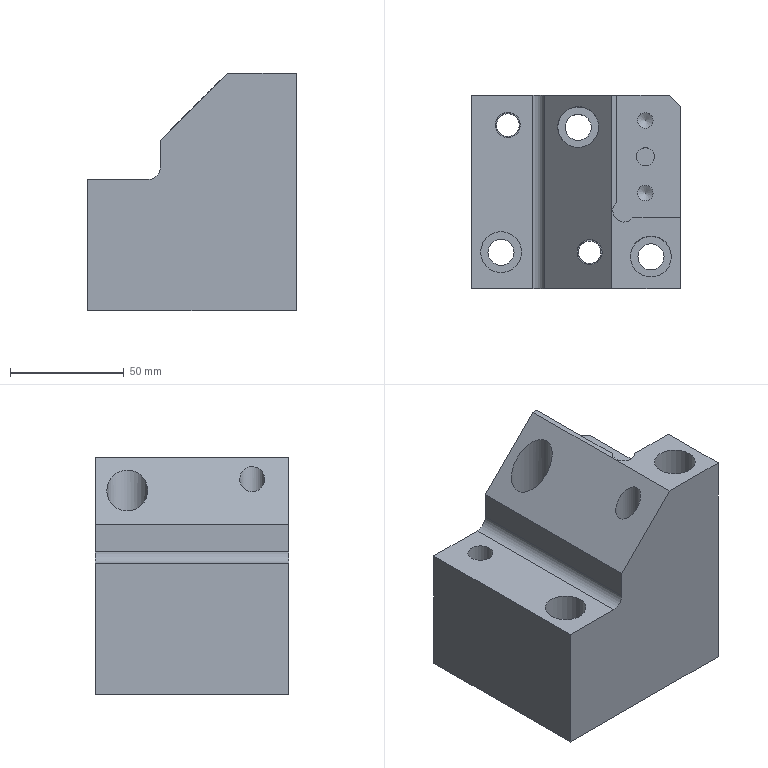Part | NX | features solid 2 | 1 solid | 36 faces | box 92 x 85 x 104.5 mm | volume 547105 mm3 | plane 19 | cylinder 15 | cone 2 | commonest cylinder face diameters 11.5 x3 6.8 x2 10 x2 10.001 x2 11 x2 18.008 x2
STEP:
#1=CARTESIAN_POINT('',(3692.099,-404.,-58.502));
#2=VERTEX_POINT('',#1);
#3=CARTESIAN_POINT('',(3688.699,-404.,-58.502));
#4=DIRECTION('',(0.,0.,1.));
#5=DIRECTION('',(1.,0.,0.));
#6=AXIS2_PLACEMENT_3D('',#3,#4,#5);
#7=CIRCLE('',#6,3.4);
#8=EDGE_CURVE('',#2,#2,#7,.T.);
#9=ORIENTED_EDGE('',*,*,#8,.T.);
#10=EDGE_LOOP('',(#9));
#11=FACE_BOUND('',#10,.T.);
#12=CARTESIAN_POINT('',(3688.699,-404.,-60.545));
#13=VERTEX_POINT('',#12);
#14=VERTEX_LOOP('',#13);
#15=FACE_BOUND('',#14,.T.);
#16=CARTESIAN_POINT('',(3688.699,-404.,-58.5));
#17=DIRECTION('',(0.,0.,1.));
#18=DIRECTION('',(1.,0.,0.));
#19=AXIS2_PLACEMENT_3D('',#16,#17,#18);
#20=CONICAL_SURFACE('',#19,3.403,1.03);
#21=ADVANCED_FACE('',(#11,#15),#20,.F.);
#22=ORIENTED_EDGE('',*,*,#8,.F.);
#23=EDGE_LOOP('',(#22));
#24=FACE_BOUND('',#23,.T.);
#25=CARTESIAN_POINT('',(3685.299,-404.,-33.5));
#26=VERTEX_POINT('',#25);
#27=CARTESIAN_POINT('',(3688.699,-404.,-33.5));
#28=DIRECTION('',(0.,0.,1.));
#29=DIRECTION('',(-1.,0.,0.));
#30=AXIS2_PLACEMENT_3D('',#27,#28,#29);
#31=CIRCLE('',#30,3.4);
#32=EDGE_CURVE('',#26,#26,#31,.T.);
#33=ORIENTED_EDGE('',*,*,#32,.T.);
#34=EDGE_LOOP('',(#33));
#35=FACE_BOUND('',#34,.T.);
#36=CARTESIAN_POINT('',(3688.699,-404.,-33.5));
#37=DIRECTION('',(0.,0.,-1.));
#38=DIRECTION('',(-1.,0.,0.));
#39=AXIS2_PLACEMENT_3D('',#36,#37,#38);
#40=CYLINDRICAL_SURFACE('',#39,3.4);
#41=ADVANCED_FACE('',(#24,#35),#40,.F.);
#42=CARTESIAN_POINT('',(3659.199,-462.,-83.));
#43=VERTEX_POINT('',#42);
#44=CARTESIAN_POINT('',(3664.199,-462.,-83.));
#45=DIRECTION('',(0.,0.,1.));
#46=DIRECTION('',(-1.,0.,0.));
#47=AXIS2_PLACEMENT_3D('',#44,#45,#46);
#48=CIRCLE('',#47,5.);
#49=EDGE_CURVE('',#43,#43,#48,.T.);
#50=ORIENTED_EDGE('',*,*,#49,.F.);
#51=EDGE_LOOP('',(#50));
#52=FACE_BOUND('',#51,.T.);
#53=CARTESIAN_POINT('',(3669.699,-462.,-83.));
#54=VERTEX_POINT('',#53);
#55=CARTESIAN_POINT('',(3664.199,-462.,-83.));
#56=DIRECTION('',(0.,0.,1.));
#57=DIRECTION('',(1.,0.,0.));
#58=AXIS2_PLACEMENT_3D('',#55,#56,#57);
#59=CIRCLE('',#58,5.5);
#60=EDGE_CURVE('',#54,#54,#59,.T.);
#61=ORIENTED_EDGE('',*,*,#60,.T.);
#62=EDGE_LOOP('',(#61));
#63=FACE_BOUND('',#62,.T.);
#64=CARTESIAN_POINT('',(3691.199,-464.,-83.));
#65=DIRECTION('',(0.,0.,-1.));
#66=DIRECTION('',(-1.,0.,0.));
#67=AXIS2_PLACEMENT_3D('',#64,#65,#66);
#68=PLANE('',#67);
#69=ADVANCED_FACE('',(#52,#63),#68,.F.);
#70=CARTESIAN_POINT('',(3682.199,-464.,-83.));
#71=VERTEX_POINT('',#70);
#72=CARTESIAN_POINT('',(3691.199,-464.,-83.));
#73=DIRECTION('',(0.,0.,-1.));
#74=DIRECTION('',(-1.,0.,0.));
#75=AXIS2_PLACEMENT_3D('',#72,#73,#74);
#76=CIRCLE('',#75,9.);
#77=EDGE_CURVE('',#71,#71,#76,.T.);
#78=ORIENTED_EDGE('',*,*,#77,.F.);
#79=EDGE_LOOP('',(#78));
#80=FACE_BOUND('',#79,.T.);
#81=CARTESIAN_POINT('',(3685.449,-464.,-83.));
#82=VERTEX_POINT('',#81);
#83=CARTESIAN_POINT('',(3691.199,-464.,-83.));
#84=DIRECTION('',(0.,0.,-1.));
#85=DIRECTION('',(-1.,0.,0.));
#86=AXIS2_PLACEMENT_3D('',#83,#84,#85);
#87=CIRCLE('',#86,5.75);
#88=EDGE_CURVE('',#82,#82,#87,.T.);
#89=ORIENTED_EDGE('',*,*,#88,.T.);
#90=EDGE_LOOP('',(#89));
#91=FACE_BOUND('',#90,.T.);
#92=CARTESIAN_POINT('',(2606.199,-221.,-83.));
#93=DIRECTION('',(0.,0.,-1.));
#94=DIRECTION('',(-1.,0.,0.));
#95=AXIS2_PLACEMENT_3D('',#92,#93,#94);
#96=PLANE('',#95);
#97=ADVANCED_FACE('',(#80,#91),#96,.F.);
#98=CARTESIAN_POINT('',(3650.195,-407.,-83.));
#99=VERTEX_POINT('',#98);
#100=CARTESIAN_POINT('',(3659.199,-407.,-83.));
#101=DIRECTION('',(0.,0.,-1.));
#102=DIRECTION('',(-1.,0.,0.));
#103=AXIS2_PLACEMENT_3D('',#100,#101,#102);
#104=CIRCLE('',#103,9.004);
#105=EDGE_CURVE('',#99,#99,#104,.T.);
#106=ORIENTED_EDGE('',*,*,#105,.F.);
#107=EDGE_LOOP('',(#106));
#108=FACE_BOUND('',#107,.T.);
#109=CARTESIAN_POINT('',(3653.449,-407.,-83.));
#110=VERTEX_POINT('',#109);
#111=CARTESIAN_POINT('',(3659.199,-407.,-83.));
#112=DIRECTION('',(0.,0.,-1.));
#113=DIRECTION('',(-1.,0.,0.));
#114=AXIS2_PLACEMENT_3D('',#111,#112,#113);
#115=CIRCLE('',#114,5.75);
#116=EDGE_CURVE('',#110,#110,#115,.T.);
#117=ORIENTED_EDGE('',*,*,#116,.T.);
#118=EDGE_LOOP('',(#117));
#119=FACE_BOUND('',#118,.T.);
#120=CARTESIAN_POINT('',(2606.199,-221.,-83.));
#121=DIRECTION('',(0.,0.,-1.));
#122=DIRECTION('',(-1.,0.,0.));
#123=AXIS2_PLACEMENT_3D('',#120,#121,#122);
#124=PLANE('',#123);
#125=ADVANCED_FACE('',(#108,#119),#124,.F.);
#126=CARTESIAN_POINT('',(3623.199,-406.,-83.));
#127=VERTEX_POINT('',#126);
#128=CARTESIAN_POINT('',(3628.199,-406.,-83.));
#129=DIRECTION('',(0.,0.,1.));
#130=DIRECTION('',(-1.,0.,0.));
#131=AXIS2_PLACEMENT_3D('',#128,#129,#130);
#132=CIRCLE('',#131,5.);
#133=EDGE_CURVE('',#127,#127,#132,.T.);
#134=ORIENTED_EDGE('',*,*,#133,.F.);
#135=EDGE_LOOP('',(#134));
#136=FACE_BOUND('',#135,.T.);
#137=CARTESIAN_POINT('',(3633.699,-406.,-83.));
#138=VERTEX_POINT('',#137);
#139=CARTESIAN_POINT('',(3628.199,-406.,-83.));
#140=DIRECTION('',(0.,0.,1.));
#141=DIRECTION('',(1.,0.,0.));
#142=AXIS2_PLACEMENT_3D('',#139,#140,#141);
#143=CIRCLE('',#142,5.5);
#144=EDGE_CURVE('',#138,#138,#143,.T.);
#145=ORIENTED_EDGE('',*,*,#144,.T.);
#146=EDGE_LOOP('',(#145));
#147=FACE_BOUND('',#146,.T.);
#148=CARTESIAN_POINT('',(3660.199,-443.,-83.));
#149=DIRECTION('',(0.,0.,-1.));
#150=DIRECTION('',(-1.,0.,0.));
#151=AXIS2_PLACEMENT_3D('',#148,#149,#150);
#152=PLANE('',#151);
#153=ADVANCED_FACE('',(#136,#147),#152,.F.);
#154=CARTESIAN_POINT('',(3616.195,-462.,-83.));
#155=VERTEX_POINT('',#154);
#156=CARTESIAN_POINT('',(3625.199,-462.,-83.));
#157=DIRECTION('',(0.,0.,-1.));
#158=DIRECTION('',(-1.,0.,0.));
#159=AXIS2_PLACEMENT_3D('',#156,#157,#158);
#160=CIRCLE('',#159,9.004);
#161=EDGE_CURVE('',#155,#155,#160,.T.);
#162=ORIENTED_EDGE('',*,*,#161,.F.);
#163=EDGE_LOOP('',(#162));
#164=FACE_BOUND('',#163,.T.);
#165=CARTESIAN_POINT('',(3619.449,-462.,-83.));
#166=VERTEX_POINT('',#165);
#167=CARTESIAN_POINT('',(3625.199,-462.,-83.));
#168=DIRECTION('',(0.,0.,-1.));
#169=DIRECTION('',(-1.,0.,0.));
#170=AXIS2_PLACEMENT_3D('',#167,#168,#169);
#171=CIRCLE('',#170,5.75);
#172=EDGE_CURVE('',#166,#166,#171,.T.);
#173=ORIENTED_EDGE('',*,*,#172,.T.);
#174=EDGE_LOOP('',(#173));
#175=FACE_BOUND('',#174,.T.);
#176=CARTESIAN_POINT('',(2606.199,-238.,-83.));
#177=DIRECTION('',(0.,0.,-1.));
#178=DIRECTION('',(-1.,0.,0.));
#179=AXIS2_PLACEMENT_3D('',#176,#177,#178);
#180=PLANE('',#179);
#181=ADVANCED_FACE('',(#164,#175),#180,.F.);
#182=CARTESIAN_POINT('',(3616.195,-462.,-55.16));
#183=VERTEX_POINT('',#182);
#184=CARTESIAN_POINT('',(3625.199,-462.,-55.16));
#185=DIRECTION('',(0.,0.,-1.));
#186=DIRECTION('',(-1.,0.,0.));
#187=AXIS2_PLACEMENT_3D('',#184,#185,#186);
#188=CIRCLE('',#187,9.004);
#189=EDGE_CURVE('',#183,#183,#188,.T.);
#190=ORIENTED_EDGE('',*,*,#189,.F.);
#191=EDGE_LOOP('',(#190));
#192=FACE_BOUND('',#191,.T.);
#193=ORIENTED_EDGE('',*,*,#161,.T.);
#194=EDGE_LOOP('',(#193));
#195=FACE_BOUND('',#194,.T.);
#196=CARTESIAN_POINT('',(3625.199,-462.,-8.5));
#197=DIRECTION('',(0.,0.,-1.));
#198=DIRECTION('',(1.,0.,0.));
#199=AXIS2_PLACEMENT_3D('',#196,#197,#198);
#200=CYLINDRICAL_SURFACE('',#199,9.004);
#201=ADVANCED_FACE('',(#192,#195),#200,.F.);
#202=CARTESIAN_POINT('',(3622.699,-406.,-55.16));
#203=VERTEX_POINT('',#202);
#204=CARTESIAN_POINT('',(3628.199,-406.,-55.16));
#205=DIRECTION('',(0.,0.,1.));
#206=DIRECTION('',(-1.,0.,0.));
#207=AXIS2_PLACEMENT_3D('',#204,#205,#206);
#208=CIRCLE('',#207,5.5);
#209=EDGE_CURVE('',#203,#203,#208,.T.);
#210=ORIENTED_EDGE('',*,*,#209,.T.);
#211=EDGE_LOOP('',(#210));
#212=FACE_BOUND('',#211,.T.);
#213=ORIENTED_EDGE('',*,*,#144,.F.);
#214=EDGE_LOOP('',(#213));
#215=FACE_BOUND('',#214,.T.);
#216=CARTESIAN_POINT('',(3628.199,-406.,66.5));
#217=DIRECTION('',(0.,0.,-1.));
#218=DIRECTION('',(-1.,0.,0.));
#219=AXIS2_PLACEMENT_3D('',#216,#217,#218);
#220=CYLINDRICAL_SURFACE('',#219,5.5);
#221=ADVANCED_FACE('',(#212,#215),#220,.F.);
#222=ORIENTED_EDGE('',*,*,#105,.T.);
#223=EDGE_LOOP('',(#222));
#224=FACE_BOUND('',#223,.T.);
#225=CARTESIAN_POINT('',(3650.195,-407.,-32.133));
#226=VERTEX_POINT('',#225);
#227=CARTESIAN_POINT('',(3659.199,-407.,-23.129));
#228=DIRECTION('',(-0.7071,0.,0.7071));
#229=DIRECTION('',(-0.7071,0.,-0.7071));
#230=AXIS2_PLACEMENT_3D('',#227,#228,#229);
#231=ELLIPSE('',#230,12.734,9.004);
#232=EDGE_CURVE('',#226,#226,#231,.T.);
#233=ORIENTED_EDGE('',*,*,#232,.T.);
#234=EDGE_LOOP('',(#233));
#235=FACE_BOUND('',#234,.T.);
#236=CARTESIAN_POINT('',(3659.199,-407.,-8.5));
#237=DIRECTION('',(0.,0.,-1.));
#238=DIRECTION('',(1.,0.,0.));
#239=AXIS2_PLACEMENT_3D('',#236,#237,#238);
#240=CYLINDRICAL_SURFACE('',#239,9.004);
#241=ADVANCED_FACE('',(#224,#235),#240,.F.);
#242=ORIENTED_EDGE('',*,*,#60,.F.);
#243=EDGE_LOOP('',(#242));
#244=FACE_BOUND('',#243,.T.);
#245=CARTESIAN_POINT('',(3658.699,-462.,-23.629));
#246=VERTEX_POINT('',#245);
#247=CARTESIAN_POINT('',(3664.199,-462.,-18.129));
#248=DIRECTION('',(-0.7071,0.,0.7071));
#249=DIRECTION('',(-0.7071,0.,-0.7071));
#250=AXIS2_PLACEMENT_3D('',#247,#248,#249);
#251=ELLIPSE('',#250,7.778,5.5);
#252=EDGE_CURVE('',#246,#246,#251,.T.);
#253=ORIENTED_EDGE('',*,*,#252,.T.);
#254=EDGE_LOOP('',(#253));
#255=FACE_BOUND('',#254,.T.);
#256=CARTESIAN_POINT('',(3664.199,-462.,66.5));
#257=DIRECTION('',(0.,0.,-1.));
#258=DIRECTION('',(-1.,0.,0.));
#259=AXIS2_PLACEMENT_3D('',#256,#257,#258);
#260=CYLINDRICAL_SURFACE('',#259,5.5);
#261=ADVANCED_FACE('',(#244,#255),#260,.F.);
#262=ORIENTED_EDGE('',*,*,#77,.T.);
#263=EDGE_LOOP('',(#262));
#264=FACE_BOUND('',#263,.T.);
#265=CARTESIAN_POINT('',(3700.199,-464.,-8.5));
#266=VERTEX_POINT('',#265);
#267=CARTESIAN_POINT('',(3691.199,-464.,-8.5));
#268=DIRECTION('',(0.,0.,-1.));
#269=DIRECTION('',(1.,0.,0.));
#270=AXIS2_PLACEMENT_3D('',#267,#268,#269);
#271=CIRCLE('',#270,9.);
#272=EDGE_CURVE('',#266,#266,#271,.T.);
#273=ORIENTED_EDGE('',*,*,#272,.F.);
#274=EDGE_LOOP('',(#273));
#275=FACE_BOUND('',#274,.T.);
#276=CARTESIAN_POINT('',(3691.199,-464.,-8.5));
#277=DIRECTION('',(0.,0.,-1.));
#278=DIRECTION('',(1.,0.,0.));
#279=AXIS2_PLACEMENT_3D('',#276,#277,#278);
#280=CYLINDRICAL_SURFACE('',#279,9.);
#281=ADVANCED_FACE('',(#264,#275),#280,.F.);
#282=CARTESIAN_POINT('',(3659.199,-462.,-113.));
#283=VERTEX_POINT('',#282);
#284=CARTESIAN_POINT('',(3664.199,-462.,-113.));
#285=DIRECTION('',(0.,0.,1.));
#286=DIRECTION('',(-1.,0.,0.));
#287=AXIS2_PLACEMENT_3D('',#284,#285,#286);
#288=CIRCLE('',#287,5.);
#289=EDGE_CURVE('',#283,#283,#288,.T.);
#290=ORIENTED_EDGE('',*,*,#289,.F.);
#291=EDGE_LOOP('',(#290));
#292=FACE_BOUND('',#291,.T.);
#293=ORIENTED_EDGE('',*,*,#49,.T.);
#294=EDGE_LOOP('',(#293));
#295=FACE_BOUND('',#294,.T.);
#296=CARTESIAN_POINT('',(3664.199,-462.,67.));
#297=DIRECTION('',(0.,0.,-1.));
#298=DIRECTION('',(-1.,0.,0.));
#299=AXIS2_PLACEMENT_3D('',#296,#297,#298);
#300=CYLINDRICAL_SURFACE('',#299,5.);
#301=ADVANCED_FACE('',(#292,#295),#300,.F.);
#302=CARTESIAN_POINT('',(3685.449,-464.,-113.));
#303=VERTEX_POINT('',#302);
#304=CARTESIAN_POINT('',(3691.199,-464.,-113.));
#305=DIRECTION('',(0.,0.,-1.));
#306=DIRECTION('',(-1.,0.,0.));
#307=AXIS2_PLACEMENT_3D('',#304,#305,#306);
#308=CIRCLE('',#307,5.75);
#309=EDGE_CURVE('',#303,#303,#308,.T.);
#310=ORIENTED_EDGE('',*,*,#309,.T.);
#311=EDGE_LOOP('',(#310));
#312=FACE_BOUND('',#311,.T.);
#313=ORIENTED_EDGE('',*,*,#88,.F.);
#314=EDGE_LOOP('',(#313));
#315=FACE_BOUND('',#314,.T.);
#316=CARTESIAN_POINT('',(3691.199,-464.,-6.));
#317=DIRECTION('',(0.,0.,-1.));
#318=DIRECTION('',(1.,0.,0.));
#319=AXIS2_PLACEMENT_3D('',#316,#317,#318);
#320=CYLINDRICAL_SURFACE('',#319,5.75);
#321=ADVANCED_FACE('',(#312,#315),#320,.F.);
#322=CARTESIAN_POINT('',(3653.449,-407.,-113.));
#323=VERTEX_POINT('',#322);
#324=CARTESIAN_POINT('',(3659.199,-407.,-113.));
#325=DIRECTION('',(0.,0.,-1.));
#326=DIRECTION('',(-1.,0.,0.));
#327=AXIS2_PLACEMENT_3D('',#324,#325,#326);
#328=CIRCLE('',#327,5.75);
#329=EDGE_CURVE('',#323,#323,#328,.T.);
#330=ORIENTED_EDGE('',*,*,#329,.T.);
#331=EDGE_LOOP('',(#330));
#332=FACE_BOUND('',#331,.T.);
#333=ORIENTED_EDGE('',*,*,#116,.F.);
#334=EDGE_LOOP('',(#333));
#335=FACE_BOUND('',#334,.T.);
#336=CARTESIAN_POINT('',(3659.199,-407.,-6.));
#337=DIRECTION('',(0.,0.,-1.));
#338=DIRECTION('',(1.,0.,0.));
#339=AXIS2_PLACEMENT_3D('',#336,#337,#338);
#340=CYLINDRICAL_SURFACE('',#339,5.75);
#341=ADVANCED_FACE('',(#332,#335),#340,.F.);
#342=CARTESIAN_POINT('',(3623.199,-406.,-113.));
#343=VERTEX_POINT('',#342);
#344=CARTESIAN_POINT('',(3628.199,-406.,-113.));
#345=DIRECTION('',(0.,0.,1.));
#346=DIRECTION('',(-1.,0.,0.));
#347=AXIS2_PLACEMENT_3D('',#344,#345,#346);
#348=CIRCLE('',#347,5.);
#349=EDGE_CURVE('',#343,#343,#348,.T.);
#350=ORIENTED_EDGE('',*,*,#349,.F.);
#351=EDGE_LOOP('',(#350));
#352=FACE_BOUND('',#351,.T.);
#353=ORIENTED_EDGE('',*,*,#133,.T.);
#354=EDGE_LOOP('',(#353));
#355=FACE_BOUND('',#354,.T.);
#356=CARTESIAN_POINT('',(3628.199,-406.,67.));
#357=DIRECTION('',(0.,0.,-1.));
#358=DIRECTION('',(-1.,0.,0.));
#359=AXIS2_PLACEMENT_3D('',#356,#357,#358);
#360=CYLINDRICAL_SURFACE('',#359,5.);
#361=ADVANCED_FACE('',(#352,#355),#360,.F.);
#362=CARTESIAN_POINT('',(3619.449,-462.,-113.));
#363=VERTEX_POINT('',#362);
#364=CARTESIAN_POINT('',(3625.199,-462.,-113.));
#365=DIRECTION('',(0.,0.,-1.));
#366=DIRECTION('',(-1.,0.,0.));
#367=AXIS2_PLACEMENT_3D('',#364,#365,#366);
#368=CIRCLE('',#367,5.75);
#369=EDGE_CURVE('',#363,#363,#368,.T.);
#370=ORIENTED_EDGE('',*,*,#369,.T.);
#371=EDGE_LOOP('',(#370));
#372=FACE_BOUND('',#371,.T.);
#373=ORIENTED_EDGE('',*,*,#172,.F.);
#374=EDGE_LOOP('',(#373));
#375=FACE_BOUND('',#374,.T.);
#376=CARTESIAN_POINT('',(3625.199,-462.,-6.));
#377=DIRECTION('',(0.,0.,-1.));
#378=DIRECTION('',(1.,0.,0.));
#379=AXIS2_PLACEMENT_3D('',#376,#377,#378);
#380=CYLINDRICAL_SURFACE('',#379,5.75);
#381=ADVANCED_FACE('',(#372,#375),#380,.F.);
#382=CARTESIAN_POINT('',(3692.099,-436.,-58.502));
#383=VERTEX_POINT('',#382);
#384=CARTESIAN_POINT('',(3688.699,-436.,-58.502));
#385=DIRECTION('',(0.,0.,1.));
#386=DIRECTION('',(1.,0.,0.));
#387=AXIS2_PLACEMENT_3D('',#384,#385,#386);
#388=CIRCLE('',#387,3.4);
#389=EDGE_CURVE('',#383,#383,#388,.T.);
#390=ORIENTED_EDGE('',*,*,#389,.T.);
#391=EDGE_LOOP('',(#390));
#392=FACE_BOUND('',#391,.T.);
#393=CARTESIAN_POINT('',(3688.699,-436.,-60.545));
#394=VERTEX_POINT('',#393);
#395=VERTEX_LOOP('',#394);
#396=FACE_BOUND('',#395,.T.);
#397=CARTESIAN_POINT('',(3688.699,-436.,-58.5));
#398=DIRECTION('',(0.,0.,1.));
#399=DIRECTION('',(1.,0.,0.));
#400=AXIS2_PLACEMENT_3D('',#397,#398,#399);
#401=CONICAL_SURFACE('',#400,3.403,1.03);
#402=ADVANCED_FACE('',(#392,#396),#401,.F.);
#403=CARTESIAN_POINT('',(3612.199,-478.,-55.16));
#404=VERTEX_POINT('',#403);
#405=CARTESIAN_POINT('',(3612.199,-393.,-55.16));
#406=VERTEX_POINT('',#405);
#407=CARTESIAN_POINT('',(3612.199,-407.5,-55.16));
#408=DIRECTION('',(0.,1.,0.));
#409=VECTOR('',#408,1000.);
#410=LINE('',#407,#409);
#411=EDGE_CURVE('',#404,#406,#410,.T.);
#412=ORIENTED_EDGE('',*,*,#411,.T.);
#413=CARTESIAN_POINT('',(3612.199,-393.,-113.));
#414=VERTEX_POINT('',#413);
#415=CARTESIAN_POINT('',(3612.199,-393.,-148.5));
#416=DIRECTION('',(0.,0.,-1.));
#417=VECTOR('',#416,1000.);
#418=LINE('',#415,#417);
#419=EDGE_CURVE('',#406,#414,#418,.T.);
#420=ORIENTED_EDGE('',*,*,#419,.T.);
#421=CARTESIAN_POINT('',(3612.199,-478.,-113.));
#422=VERTEX_POINT('',#421);
#423=CARTESIAN_POINT('',(3612.199,-407.5,-113.));
#424=DIRECTION('',(0.,-1.,0.));
#425=VECTOR('',#424,1000.);
#426=LINE('',#423,#425);
#427=EDGE_CURVE('',#414,#422,#426,.T.);
#428=ORIENTED_EDGE('',*,*,#427,.T.);
#429=CARTESIAN_POINT('',(3612.199,-478.,-148.5));
#430=DIRECTION('',(0.,0.,1.));
#431=VECTOR('',#430,1000.);
#432=LINE('',#429,#431);
#433=EDGE_CURVE('',#422,#404,#432,.T.);
#434=ORIENTED_EDGE('',*,*,#433,.T.);
#435=EDGE_LOOP('',(#412,#420,#428,#434));
#436=FACE_BOUND('',#435,.T.);
#437=CARTESIAN_POINT('',(3612.199,-407.5,-148.5));
#438=DIRECTION('',(-1.,0.,0.));
#439=DIRECTION('',(0.,0.,1.));
#440=AXIS2_PLACEMENT_3D('',#437,#438,#439);
#441=PLANE('',#440);
#442=ADVANCED_FACE('',(#436),#441,.T.);
#443=ORIENTED_EDGE('',*,*,#209,.F.);
#444=EDGE_LOOP('',(#443));
#445=FACE_BOUND('',#444,.T.);
#446=ORIENTED_EDGE('',*,*,#189,.T.);
#447=EDGE_LOOP('',(#446));
#448=FACE_BOUND('',#447,.T.);
#449=CARTESIAN_POINT('',(3639.199,-478.,-55.16));
#450=VERTEX_POINT('',#449);
#451=CARTESIAN_POINT('',(3678.699,-478.,-55.16));
#452=DIRECTION('',(1.,0.,0.));
#453=VECTOR('',#452,1000.);
#454=LINE('',#451,#453);
#455=EDGE_CURVE('',#404,#450,#454,.T.);
#456=ORIENTED_EDGE('',*,*,#455,.T.);
#457=CARTESIAN_POINT('',(3639.199,-393.,-55.16));
#458=VERTEX_POINT('',#457);
#459=CARTESIAN_POINT('',(3639.199,-407.5,-55.16));
#460=DIRECTION('',(0.,1.,0.));
#461=VECTOR('',#460,1000.);
#462=LINE('',#459,#461);
#463=EDGE_CURVE('',#450,#458,#462,.T.);
#464=ORIENTED_EDGE('',*,*,#463,.T.);
#465=CARTESIAN_POINT('',(3678.699,-393.,-55.16));
#466=DIRECTION('',(-1.,0.,0.));
#467=VECTOR('',#466,1000.);
#468=LINE('',#465,#467);
#469=EDGE_CURVE('',#458,#406,#468,.T.);
#470=ORIENTED_EDGE('',*,*,#469,.T.);
#471=ORIENTED_EDGE('',*,*,#411,.F.);
#472=EDGE_LOOP('',(#456,#464,#470,#471));
#473=FACE_BOUND('',#472,.T.);
#474=CARTESIAN_POINT('',(3644.199,-407.5,-55.16));
#475=DIRECTION('',(0.,0.,-1.));
#476=DIRECTION('',(0.,-1.,0.));
#477=AXIS2_PLACEMENT_3D('',#474,#475,#476);
#478=PLANE('',#477);
#479=ADVANCED_FACE('',(#445,#448,#473),#478,.F.);
#480=CARTESIAN_POINT('',(3644.199,-478.,-50.16));
#481=VERTEX_POINT('',#480);
#482=CARTESIAN_POINT('',(3639.199,-478.,-50.16));
#483=DIRECTION('',(0.,1.,0.));
#484=DIRECTION('',(0.,0.,-1.));
#485=AXIS2_PLACEMENT_3D('',#482,#483,#484);
#486=CIRCLE('',#485,5.);
#487=EDGE_CURVE('',#481,#450,#486,.T.);
#488=ORIENTED_EDGE('',*,*,#487,.F.);
#489=CARTESIAN_POINT('',(3644.199,-393.,-50.16));
#490=VERTEX_POINT('',#489);
#491=CARTESIAN_POINT('',(3644.199,-407.5,-50.16));
#492=DIRECTION('',(0.,-1.,0.));
#493=VECTOR('',#492,1000.);
#494=LINE('',#491,#493);
#495=EDGE_CURVE('',#490,#481,#494,.T.);
#496=ORIENTED_EDGE('',*,*,#495,.F.);
#497=CARTESIAN_POINT('',(3639.199,-393.,-50.16));
#498=DIRECTION('',(0.,-1.,0.));
#499=DIRECTION('',(0.,0.,1.));
#500=AXIS2_PLACEMENT_3D('',#497,#498,#499);
#501=CIRCLE('',#500,5.);
#502=EDGE_CURVE('',#458,#490,#501,.T.);
#503=ORIENTED_EDGE('',*,*,#502,.F.);
#504=ORIENTED_EDGE('',*,*,#463,.F.);
#505=EDGE_LOOP('',(#488,#496,#503,#504));
#506=FACE_BOUND('',#505,.T.);
#507=CARTESIAN_POINT('',(3639.199,-407.5,-50.16));
#508=DIRECTION('',(0.,1.,0.));
#509=DIRECTION('',(0.,0.,1.));
#510=AXIS2_PLACEMENT_3D('',#507,#508,#509);
#511=CYLINDRICAL_SURFACE('',#510,5.);
#512=ADVANCED_FACE('',(#506),#511,.F.);
#513=CARTESIAN_POINT('',(3644.199,-393.,-38.129));
#514=VERTEX_POINT('',#513);
#515=CARTESIAN_POINT('',(3644.199,-478.,-38.129));
#516=VERTEX_POINT('',#515);
#517=CARTESIAN_POINT('',(3644.199,-407.5,-38.129));
#518=DIRECTION('',(0.,-1.,0.));
#519=VECTOR('',#518,1000.);
#520=LINE('',#517,#519);
#521=EDGE_CURVE('',#514,#516,#520,.T.);
#522=ORIENTED_EDGE('',*,*,#521,.F.);
#523=CARTESIAN_POINT('',(3644.199,-393.,-148.5));
#524=DIRECTION('',(0.,0.,1.));
#525=VECTOR('',#524,1000.);
#526=LINE('',#523,#525);
#527=EDGE_CURVE('',#490,#514,#526,.T.);
#528=ORIENTED_EDGE('',*,*,#527,.F.);
#529=ORIENTED_EDGE('',*,*,#495,.T.);
#530=CARTESIAN_POINT('',(3644.199,-478.,-148.5));
#531=DIRECTION('',(0.,0.,1.));
#532=VECTOR('',#531,1000.);
#533=LINE('',#530,#532);
#534=EDGE_CURVE('',#481,#516,#533,.T.);
#535=ORIENTED_EDGE('',*,*,#534,.T.);
#536=EDGE_LOOP('',(#522,#528,#529,#535));
#537=FACE_BOUND('',#536,.T.);
#538=CARTESIAN_POINT('',(3644.199,-407.5,-148.5));
#539=DIRECTION('',(-1.,0.,0.));
#540=DIRECTION('',(0.,0.,1.));
#541=AXIS2_PLACEMENT_3D('',#538,#539,#540);
#542=PLANE('',#541);
#543=ADVANCED_FACE('',(#537),#542,.T.);
#544=ORIENTED_EDGE('',*,*,#252,.F.);
#545=EDGE_LOOP('',(#544));
#546=FACE_BOUND('',#545,.T.);
#547=CARTESIAN_POINT('',(3673.828,-478.,-8.5));
#548=VERTEX_POINT('',#547);
#549=CARTESIAN_POINT('',(3673.828,-393.,-8.5));
#550=VERTEX_POINT('',#549);
#551=CARTESIAN_POINT('',(3673.828,-383.325,-8.5));
#552=DIRECTION('',(0.,1.,0.));
#553=VECTOR('',#552,1000.);
#554=LINE('',#551,#553);
#555=EDGE_CURVE('',#548,#550,#554,.T.);
#556=ORIENTED_EDGE('',*,*,#555,.T.);
#557=CARTESIAN_POINT('',(3672.414,-393.,-9.914));
#558=DIRECTION('',(0.7071,0.,0.7071));
#559=VECTOR('',#558,1000.);
#560=LINE('',#557,#559);
#561=EDGE_CURVE('',#514,#550,#560,.T.);
#562=ORIENTED_EDGE('',*,*,#561,.F.);
#563=ORIENTED_EDGE('',*,*,#521,.T.);
#564=CARTESIAN_POINT('',(3672.414,-478.,-9.914));
#565=DIRECTION('',(-0.7071,0.,-0.7071));
#566=VECTOR('',#565,1000.);
#567=LINE('',#564,#566);
#568=EDGE_CURVE('',#548,#516,#567,.T.);
#569=ORIENTED_EDGE('',*,*,#568,.F.);
#570=EDGE_LOOP('',(#556,#562,#563,#569));
#571=FACE_BOUND('',#570,.T.);
#572=ORIENTED_EDGE('',*,*,#232,.F.);
#573=EDGE_LOOP('',(#572));
#574=FACE_BOUND('',#573,.T.);
#575=CARTESIAN_POINT('',(3672.414,-395.489,-9.914));
#576=DIRECTION('',(-0.7071,0.,0.7071));
#577=DIRECTION('',(0.,-1.,0.));
#578=AXIS2_PLACEMENT_3D('',#575,#576,#577);
#579=PLANE('',#578);
#580=ADVANCED_FACE('',(#546,#571,#574),#579,.T.);
#581=ORIENTED_EDGE('',*,*,#272,.T.);
#582=EDGE_LOOP('',(#581));
#583=FACE_BOUND('',#582,.T.);
#584=CARTESIAN_POINT('',(3676.199,-393.,-8.5));
#585=VERTEX_POINT('',#584);
#586=CARTESIAN_POINT('',(3678.699,-393.,-8.5));
#587=DIRECTION('',(1.,0.,0.));
#588=VECTOR('',#587,1000.);
#589=LINE('',#586,#588);
#590=EDGE_CURVE('',#550,#585,#589,.T.);
#591=ORIENTED_EDGE('',*,*,#590,.F.);
#592=ORIENTED_EDGE('',*,*,#555,.F.);
#593=CARTESIAN_POINT('',(3704.199,-478.,-8.5));
#594=VERTEX_POINT('',#593);
#595=CARTESIAN_POINT('',(3678.699,-478.,-8.5));
#596=DIRECTION('',(-1.,0.,0.));
#597=VECTOR('',#596,1000.);
#598=LINE('',#595,#597);
#599=EDGE_CURVE('',#594,#548,#598,.T.);
#600=ORIENTED_EDGE('',*,*,#599,.F.);
#601=CARTESIAN_POINT('',(3704.199,-447.,-8.5));
#602=VERTEX_POINT('',#601);
#603=CARTESIAN_POINT('',(3704.199,-407.5,-8.5));
#604=DIRECTION('',(0.,-1.,0.));
#605=VECTOR('',#604,1000.);
#606=LINE('',#603,#605);
#607=EDGE_CURVE('',#602,#594,#606,.T.);
#608=ORIENTED_EDGE('',*,*,#607,.F.);
#609=CARTESIAN_POINT('',(3683.238,-447.,-8.5));
#610=VERTEX_POINT('',#609);
#611=CARTESIAN_POINT('',(3706.199,-447.,-8.5));
#612=DIRECTION('',(-1.,0.,0.));
#613=VECTOR('',#612,1000.);
#614=LINE('',#611,#613);
#615=EDGE_CURVE('',#602,#610,#614,.T.);
#616=ORIENTED_EDGE('',*,*,#615,.T.);
#617=CARTESIAN_POINT('',(3676.199,-439.961,-8.5));
#618=VERTEX_POINT('',#617);
#619=CARTESIAN_POINT('',(3679.381,-443.818,-8.5));
#620=DIRECTION('',(0.,0.,1.));
#621=DIRECTION('',(1.,0.,0.));
#622=AXIS2_PLACEMENT_3D('',#619,#620,#621);
#623=CIRCLE('',#622,5.);
#624=EDGE_CURVE('',#618,#610,#623,.T.);
#625=ORIENTED_EDGE('',*,*,#624,.F.);
#626=CARTESIAN_POINT('',(3676.199,-383.325,-8.5));
#627=DIRECTION('',(0.,-1.,0.));
#628=VECTOR('',#627,1000.);
#629=LINE('',#626,#628);
#630=EDGE_CURVE('',#585,#618,#629,.T.);
#631=ORIENTED_EDGE('',*,*,#630,.F.);
#632=EDGE_LOOP('',(#591,#592,#600,#608,#616,#625,#631));
#633=FACE_BOUND('',#632,.T.);
#634=CARTESIAN_POINT('',(2177.271,-383.325,-8.5));
#635=DIRECTION('',(0.,0.,1.));
#636=DIRECTION('',(1.,0.,0.));
#637=AXIS2_PLACEMENT_3D('',#634,#635,#636);
#638=PLANE('',#637);
#639=ADVANCED_FACE('',(#583,#633),#638,.T.);
#640=ORIENTED_EDGE('',*,*,#599,.T.);
#641=ORIENTED_EDGE('',*,*,#568,.T.);
#642=ORIENTED_EDGE('',*,*,#534,.F.);
#643=ORIENTED_EDGE('',*,*,#487,.T.);
#644=ORIENTED_EDGE('',*,*,#455,.F.);
#645=ORIENTED_EDGE('',*,*,#433,.F.);
#646=CARTESIAN_POINT('',(3704.199,-478.,-113.));
#647=VERTEX_POINT('',#646);
#648=CARTESIAN_POINT('',(3678.699,-478.,-113.));
#649=DIRECTION('',(1.,0.,0.));
#650=VECTOR('',#649,1000.);
#651=LINE('',#648,#650);
#652=EDGE_CURVE('',#422,#647,#651,.T.);
#653=ORIENTED_EDGE('',*,*,#652,.T.);
#654=CARTESIAN_POINT('',(3704.199,-478.,-148.5));
#655=DIRECTION('',(0.,0.,1.));
#656=VECTOR('',#655,1000.);
#657=LINE('',#654,#656);
#658=EDGE_CURVE('',#647,#594,#657,.T.);
#659=ORIENTED_EDGE('',*,*,#658,.T.);
#660=EDGE_LOOP('',(#640,#641,#642,#643,#644,#645,#653,#659));
#661=FACE_BOUND('',#660,.T.);
#662=CARTESIAN_POINT('',(3678.699,-478.,-148.5));
#663=DIRECTION('',(0.,-1.,0.));
#664=DIRECTION('',(0.,0.,-1.));
#665=AXIS2_PLACEMENT_3D('',#662,#663,#664);
#666=PLANE('',#665);
#667=ADVANCED_FACE('',(#661),#666,.T.);
#668=ORIENTED_EDGE('',*,*,#369,.F.);
#669=EDGE_LOOP('',(#668));
#670=FACE_BOUND('',#669,.T.);
#671=ORIENTED_EDGE('',*,*,#349,.T.);
#672=EDGE_LOOP('',(#671));
#673=FACE_BOUND('',#672,.T.);
#674=ORIENTED_EDGE('',*,*,#329,.F.);
#675=EDGE_LOOP('',(#674));
#676=FACE_BOUND('',#675,.T.);
#677=ORIENTED_EDGE('',*,*,#309,.F.);
#678=EDGE_LOOP('',(#677));
#679=FACE_BOUND('',#678,.T.);
#680=CARTESIAN_POINT('',(3699.199,-393.,-113.));
#681=VERTEX_POINT('',#680);
#682=CARTESIAN_POINT('',(3678.699,-393.,-113.));
#683=DIRECTION('',(-1.,0.,0.));
#684=VECTOR('',#683,1000.);
#685=LINE('',#682,#684);
#686=EDGE_CURVE('',#681,#414,#685,.T.);
#687=ORIENTED_EDGE('',*,*,#686,.F.);
#688=CARTESIAN_POINT('',(3704.199,-398.,-113.));
#689=VERTEX_POINT('',#688);
#690=CARTESIAN_POINT('',(3066.699,239.5,-113.));
#691=DIRECTION('',(0.7071,-0.7071,0.));
#692=VECTOR('',#691,1000.);
#693=LINE('',#690,#692);
#694=EDGE_CURVE('',#681,#689,#693,.T.);
#695=ORIENTED_EDGE('',*,*,#694,.T.);
#696=CARTESIAN_POINT('',(3704.199,-407.5,-113.));
#697=DIRECTION('',(0.,1.,0.));
#698=VECTOR('',#697,1000.);
#699=LINE('',#696,#698);
#700=EDGE_CURVE('',#647,#689,#699,.T.);
#701=ORIENTED_EDGE('',*,*,#700,.F.);
#702=ORIENTED_EDGE('',*,*,#652,.F.);
#703=ORIENTED_EDGE('',*,*,#427,.F.);
#704=EDGE_LOOP('',(#687,#695,#701,#702,#703));
#705=FACE_BOUND('',#704,.T.);
#706=ORIENTED_EDGE('',*,*,#289,.T.);
#707=EDGE_LOOP('',(#706));
#708=FACE_BOUND('',#707,.T.);
#709=CARTESIAN_POINT('',(2606.199,-221.,-113.));
#710=DIRECTION('',(0.,0.,-1.));
#711=DIRECTION('',(-1.,0.,0.));
#712=AXIS2_PLACEMENT_3D('',#709,#710,#711);
#713=PLANE('',#712);
#714=ADVANCED_FACE('',(#670,#673,#676,#679,#705,#708),#713,.T.);
#715=CARTESIAN_POINT('',(3684.699,-420.,-53.5));
#716=VERTEX_POINT('',#715);
#717=CARTESIAN_POINT('',(3688.699,-420.,-53.5));
#718=DIRECTION('',(0.,0.,1.));
#719=DIRECTION('',(-1.,0.,0.));
#720=AXIS2_PLACEMENT_3D('',#717,#718,#719);
#721=CIRCLE('',#720,4.);
#722=EDGE_CURVE('',#716,#716,#721,.T.);
#723=ORIENTED_EDGE('',*,*,#722,.T.);
#724=EDGE_LOOP('',(#723));
#725=FACE_BOUND('',#724,.T.);
#726=CARTESIAN_POINT('',(3688.699,-420.,-53.5));
#727=DIRECTION('',(0.,0.,-1.));
#728=DIRECTION('',(-1.,0.,0.));
#729=AXIS2_PLACEMENT_3D('',#726,#727,#728);
#730=PLANE('',#729);
#731=ADVANCED_FACE('',(#725),#730,.F.);
#732=ORIENTED_EDGE('',*,*,#389,.F.);
#733=EDGE_LOOP('',(#732));
#734=FACE_BOUND('',#733,.T.);
#735=CARTESIAN_POINT('',(3685.299,-436.,-33.5));
#736=VERTEX_POINT('',#735);
#737=CARTESIAN_POINT('',(3688.699,-436.,-33.5));
#738=DIRECTION('',(0.,0.,-1.));
#739=DIRECTION('',(-1.,0.,0.));
#740=AXIS2_PLACEMENT_3D('',#737,#738,#739);
#741=CIRCLE('',#740,3.4);
#742=EDGE_CURVE('',#736,#736,#741,.T.);
#743=ORIENTED_EDGE('',*,*,#742,.F.);
#744=EDGE_LOOP('',(#743));
#745=FACE_BOUND('',#744,.T.);
#746=CARTESIAN_POINT('',(3688.699,-436.,-33.5));
#747=DIRECTION('',(0.,0.,-1.));
#748=DIRECTION('',(-1.,0.,0.));
#749=AXIS2_PLACEMENT_3D('',#746,#747,#748);
#750=CYLINDRICAL_SURFACE('',#749,3.4);
#751=ADVANCED_FACE('',(#734,#745),#750,.F.);
#752=ORIENTED_EDGE('',*,*,#694,.F.);
#753=CARTESIAN_POINT('',(3699.199,-393.,-33.5));
#754=VERTEX_POINT('',#753);
#755=CARTESIAN_POINT('',(3699.199,-393.,-148.5));
#756=DIRECTION('',(0.,0.,-1.));
#757=VECTOR('',#756,1000.);
#758=LINE('',#755,#757);
#759=EDGE_CURVE('',#754,#681,#758,.T.);
#760=ORIENTED_EDGE('',*,*,#759,.F.);
#761=CARTESIAN_POINT('',(3704.199,-398.,-33.5));
#762=VERTEX_POINT('',#761);
#763=CARTESIAN_POINT('',(3704.199,-398.,-33.5));
#764=DIRECTION('',(-0.7071,0.7071,0.));
#765=VECTOR('',#764,1000.);
#766=LINE('',#763,#765);
#767=EDGE_CURVE('',#762,#754,#766,.T.);
#768=ORIENTED_EDGE('',*,*,#767,.F.);
#769=CARTESIAN_POINT('',(3704.199,-398.,-148.5));
#770=DIRECTION('',(0.,0.,1.));
#771=VECTOR('',#770,1000.);
#772=LINE('',#769,#771);
#773=EDGE_CURVE('',#689,#762,#772,.T.);
#774=ORIENTED_EDGE('',*,*,#773,.F.);
#775=EDGE_LOOP('',(#752,#760,#768,#774));
#776=FACE_BOUND('',#775,.T.);
#777=CARTESIAN_POINT('',(3704.199,-398.,-148.5));
#778=DIRECTION('',(-0.7071,-0.7071,0.));
#779=DIRECTION('',(0.,0.,-1.));
#780=AXIS2_PLACEMENT_3D('',#777,#778,#779);
#781=PLANE('',#780);
#782=ADVANCED_FACE('',(#776),#781,.F.);
#783=CARTESIAN_POINT('',(3676.199,-393.,-33.5));
#784=VERTEX_POINT('',#783);
#785=CARTESIAN_POINT('',(3678.699,-393.,-33.5));
#786=DIRECTION('',(-1.,0.,0.));
#787=VECTOR('',#786,1000.);
#788=LINE('',#785,#787);
#789=EDGE_CURVE('',#754,#784,#788,.T.);
#790=ORIENTED_EDGE('',*,*,#789,.F.);
#791=ORIENTED_EDGE('',*,*,#759,.T.);
#792=ORIENTED_EDGE('',*,*,#686,.T.);
#793=ORIENTED_EDGE('',*,*,#419,.F.);
#794=ORIENTED_EDGE('',*,*,#469,.F.);
#795=ORIENTED_EDGE('',*,*,#502,.T.);
#796=ORIENTED_EDGE('',*,*,#527,.T.);
#797=ORIENTED_EDGE('',*,*,#561,.T.);
#798=ORIENTED_EDGE('',*,*,#590,.T.);
#799=CARTESIAN_POINT('',(3676.199,-393.,-148.5));
#800=DIRECTION('',(0.,0.,1.));
#801=VECTOR('',#800,1000.);
#802=LINE('',#799,#801);
#803=EDGE_CURVE('',#784,#585,#802,.T.);
#804=ORIENTED_EDGE('',*,*,#803,.F.);
#805=EDGE_LOOP('',(#790,#791,#792,#793,#794,#795,#796,#797,#798,#804));
#806=FACE_BOUND('',#805,.T.);
#807=CARTESIAN_POINT('',(3678.699,-393.,-148.5));
#808=DIRECTION('',(0.,1.,0.));
#809=DIRECTION('',(0.,0.,1.));
#810=AXIS2_PLACEMENT_3D('',#807,#808,#809);
#811=PLANE('',#810);
#812=ADVANCED_FACE('',(#806),#811,.T.);
#813=ORIENTED_EDGE('',*,*,#803,.T.);
#814=ORIENTED_EDGE('',*,*,#630,.T.);
#815=CARTESIAN_POINT('',(3676.199,-439.961,-33.5));
#816=VERTEX_POINT('',#815);
#817=CARTESIAN_POINT('',(3676.199,-439.961,-33.5));
#818=DIRECTION('',(0.,0.,-1.));
#819=VECTOR('',#818,1000.);
#820=LINE('',#817,#819);
#821=EDGE_CURVE('',#618,#816,#820,.T.);
#822=ORIENTED_EDGE('',*,*,#821,.T.);
#823=CARTESIAN_POINT('',(3676.199,-407.5,-33.5));
#824=DIRECTION('',(0.,-1.,0.));
#825=VECTOR('',#824,1000.);
#826=LINE('',#823,#825);
#827=EDGE_CURVE('',#784,#816,#826,.T.);
#828=ORIENTED_EDGE('',*,*,#827,.F.);
#829=EDGE_LOOP('',(#813,#814,#822,#828));
#830=FACE_BOUND('',#829,.T.);
#831=CARTESIAN_POINT('',(3676.199,-407.5,-25.5));
#832=DIRECTION('',(-1.,0.,0.));
#833=DIRECTION('',(0.,0.,1.));
#834=AXIS2_PLACEMENT_3D('',#831,#832,#833);
#835=PLANE('',#834);
#836=ADVANCED_FACE('',(#830),#835,.F.);
#837=CARTESIAN_POINT('',(3683.238,-447.,-33.5));
#838=VERTEX_POINT('',#837);
#839=CARTESIAN_POINT('',(3679.381,-443.818,-33.5));
#840=DIRECTION('',(0.,0.,1.));
#841=DIRECTION('',(1.,0.,0.));
#842=AXIS2_PLACEMENT_3D('',#839,#840,#841);
#843=CIRCLE('',#842,5.);
#844=EDGE_CURVE('',#816,#838,#843,.T.);
#845=ORIENTED_EDGE('',*,*,#844,.F.);
#846=ORIENTED_EDGE('',*,*,#821,.F.);
#847=ORIENTED_EDGE('',*,*,#624,.T.);
#848=CARTESIAN_POINT('',(3683.238,-447.,-33.5));
#849=DIRECTION('',(0.,0.,1.));
#850=VECTOR('',#849,1000.);
#851=LINE('',#848,#850);
#852=EDGE_CURVE('',#838,#610,#851,.T.);
#853=ORIENTED_EDGE('',*,*,#852,.F.);
#854=EDGE_LOOP('',(#845,#846,#847,#853));
#855=FACE_BOUND('',#854,.T.);
#856=CARTESIAN_POINT('',(3679.381,-443.818,-33.5));
#857=DIRECTION('',(0.,0.,1.));
#858=DIRECTION('',(1.,0.,0.));
#859=AXIS2_PLACEMENT_3D('',#856,#857,#858);
#860=CYLINDRICAL_SURFACE('',#859,5.);
#861=ADVANCED_FACE('',(#855),#860,.F.);
#862=CARTESIAN_POINT('',(3704.199,-447.,-33.5));
#863=VERTEX_POINT('',#862);
#864=CARTESIAN_POINT('',(3706.199,-447.,-33.5));
#865=DIRECTION('',(-1.,0.,0.));
#866=VECTOR('',#865,1000.);
#867=LINE('',#864,#866);
#868=EDGE_CURVE('',#863,#838,#867,.T.);
#869=ORIENTED_EDGE('',*,*,#868,.T.);
#870=ORIENTED_EDGE('',*,*,#852,.T.);
#871=ORIENTED_EDGE('',*,*,#615,.F.);
#872=CARTESIAN_POINT('',(3704.199,-447.,-148.5));
#873=DIRECTION('',(0.,0.,-1.));
#874=VECTOR('',#873,1000.);
#875=LINE('',#872,#874);
#876=EDGE_CURVE('',#602,#863,#875,.T.);
#877=ORIENTED_EDGE('',*,*,#876,.T.);
#878=EDGE_LOOP('',(#869,#870,#871,#877));
#879=FACE_BOUND('',#878,.T.);
#880=CARTESIAN_POINT('',(3706.199,-447.,-25.5));
#881=DIRECTION('',(0.,-1.,0.));
#882=DIRECTION('',(0.,0.,-1.));
#883=AXIS2_PLACEMENT_3D('',#880,#881,#882);
#884=PLANE('',#883);
#885=ADVANCED_FACE('',(#879),#884,.F.);
#886=ORIENTED_EDGE('',*,*,#700,.T.);
#887=ORIENTED_EDGE('',*,*,#773,.T.);
#888=CARTESIAN_POINT('',(3704.199,-407.5,-33.5));
#889=DIRECTION('',(0.,1.,0.));
#890=VECTOR('',#889,1000.);
#891=LINE('',#888,#890);
#892=EDGE_CURVE('',#863,#762,#891,.T.);
#893=ORIENTED_EDGE('',*,*,#892,.F.);
#894=ORIENTED_EDGE('',*,*,#876,.F.);
#895=ORIENTED_EDGE('',*,*,#607,.T.);
#896=ORIENTED_EDGE('',*,*,#658,.F.);
#897=EDGE_LOOP('',(#886,#887,#893,#894,#895,#896));
#898=FACE_BOUND('',#897,.T.);
#899=CARTESIAN_POINT('',(3704.199,-407.5,-148.5));
#900=DIRECTION('',(1.,0.,0.));
#901=DIRECTION('',(0.,0.,-1.));
#902=AXIS2_PLACEMENT_3D('',#899,#900,#901);
#903=PLANE('',#902);
#904=ADVANCED_FACE('',(#898),#903,.T.);
#905=ORIENTED_EDGE('',*,*,#722,.F.);
#906=EDGE_LOOP('',(#905));
#907=FACE_BOUND('',#906,.T.);
#908=CARTESIAN_POINT('',(3684.699,-420.,-33.5));
#909=VERTEX_POINT('',#908);
#910=CARTESIAN_POINT('',(3688.699,-420.,-33.5));
#911=DIRECTION('',(0.,0.,-1.));
#912=DIRECTION('',(-1.,0.,0.));
#913=AXIS2_PLACEMENT_3D('',#910,#911,#912);
#914=CIRCLE('',#913,4.);
#915=EDGE_CURVE('',#909,#909,#914,.T.);
#916=ORIENTED_EDGE('',*,*,#915,.F.);
#917=EDGE_LOOP('',(#916));
#918=FACE_BOUND('',#917,.T.);
#919=CARTESIAN_POINT('',(3688.699,-420.,-53.5));
#920=DIRECTION('',(0.,0.,1.));
#921=DIRECTION('',(1.,0.,0.));
#922=AXIS2_PLACEMENT_3D('',#919,#920,#921);
#923=CYLINDRICAL_SURFACE('',#922,4.);
#924=ADVANCED_FACE('',(#907,#918),#923,.F.);
#925=ORIENTED_EDGE('',*,*,#32,.F.);
#926=EDGE_LOOP('',(#925));
#927=FACE_BOUND('',#926,.T.);
#928=ORIENTED_EDGE('',*,*,#915,.T.);
#929=EDGE_LOOP('',(#928));
#930=FACE_BOUND('',#929,.T.);
#931=ORIENTED_EDGE('',*,*,#892,.T.);
#932=ORIENTED_EDGE('',*,*,#767,.T.);
#933=ORIENTED_EDGE('',*,*,#789,.T.);
#934=ORIENTED_EDGE('',*,*,#827,.T.);
#935=ORIENTED_EDGE('',*,*,#844,.T.);
#936=ORIENTED_EDGE('',*,*,#868,.F.);
#937=EDGE_LOOP('',(#931,#932,#933,#934,#935,#936));
#938=FACE_BOUND('',#937,.T.);
#939=ORIENTED_EDGE('',*,*,#742,.T.);
#940=EDGE_LOOP('',(#939));
#941=FACE_BOUND('',#940,.T.);
#942=CARTESIAN_POINT('',(3706.199,-407.5,-33.5));
#943=DIRECTION('',(0.,0.,-1.));
#944=DIRECTION('',(-1.,0.,0.));
#945=AXIS2_PLACEMENT_3D('',#942,#943,#944);
#946=PLANE('',#945);
#947=ADVANCED_FACE('',(#927,#930,#938,#941),#946,.F.);
#948=CLOSED_SHELL('',(#21,#41,#69,#97,#125,#153,#181,#201,#221,#241,#261,#281,#301,#321,#341,#361,#381,#402,#442,#479,#512,#543,#580,#639,#667,#714,#731,#751,#782,#812,#836,#861,#885,#904,#924,#947));
#949=MANIFOLD_SOLID_BREP('',#948);
#950=(LENGTH_UNIT()NAMED_UNIT(*)SI_UNIT(.MILLI.,.METRE.));
#951=UNCERTAINTY_MEASURE_WITH_UNIT(LENGTH_MEASURE(0.00001),#950,'','');
#952=(NAMED_UNIT(*)PLANE_ANGLE_UNIT()SI_UNIT($,.RADIAN.));
#953=(NAMED_UNIT(*)SI_UNIT($,.STERADIAN.)SOLID_ANGLE_UNIT());
#954=(GEOMETRIC_REPRESENTATION_CONTEXT(3)GLOBAL_UNCERTAINTY_ASSIGNED_CONTEXT((#951))GLOBAL_UNIT_ASSIGNED_CONTEXT((#950,#952,#953))REPRESENTATION_CONTEXT('',''));
#955=ADVANCED_BREP_SHAPE_REPRESENTATION('',(#949),#954);